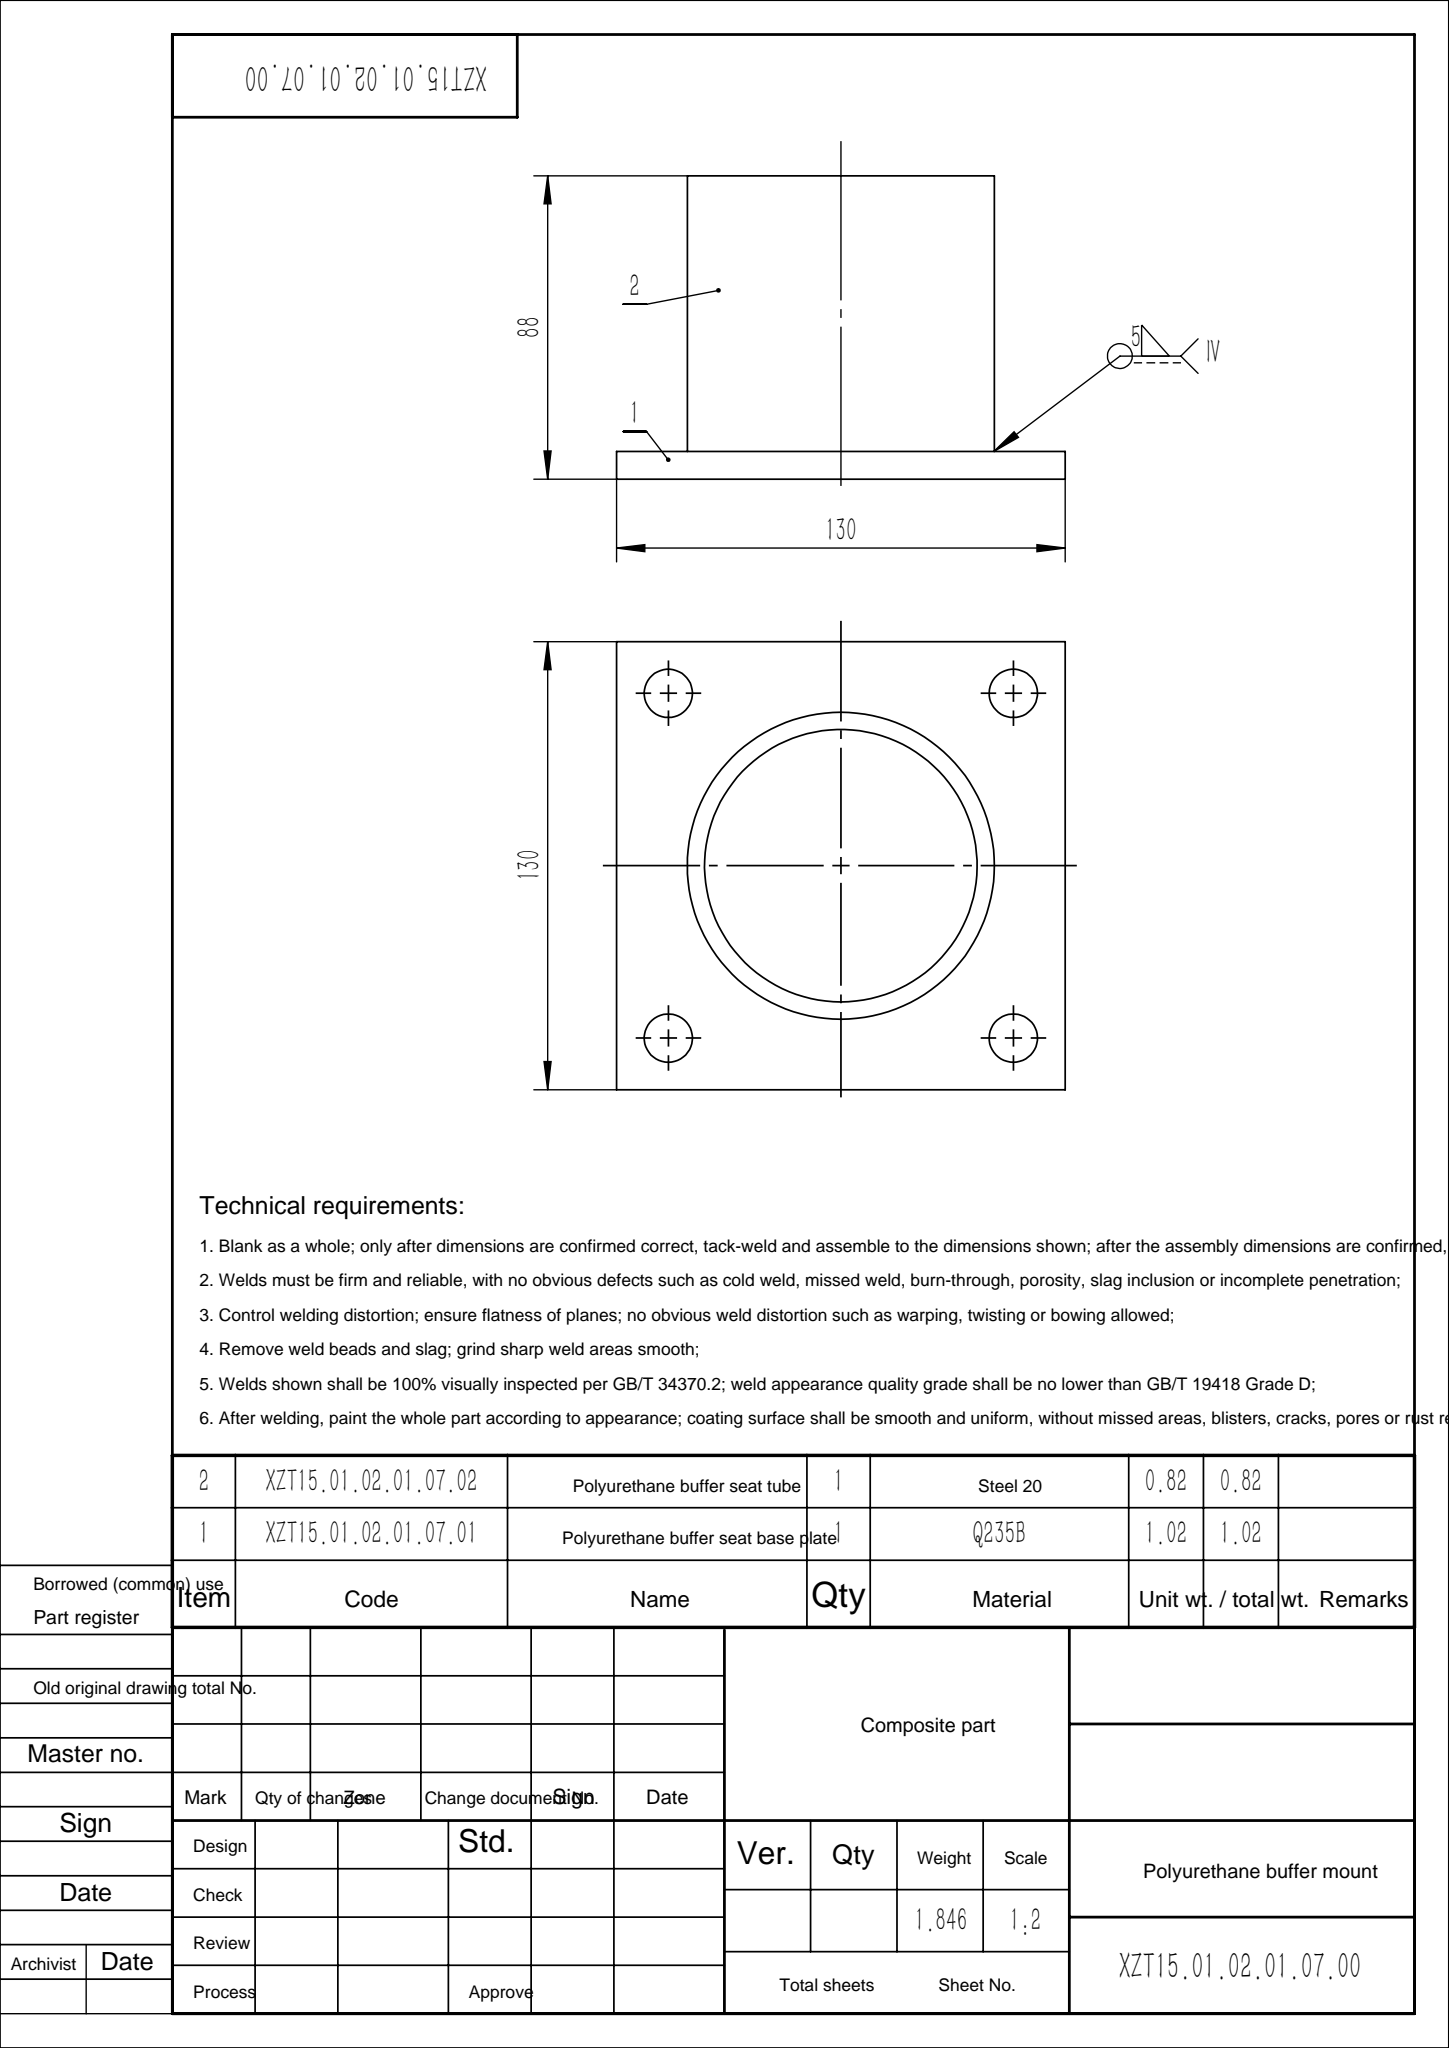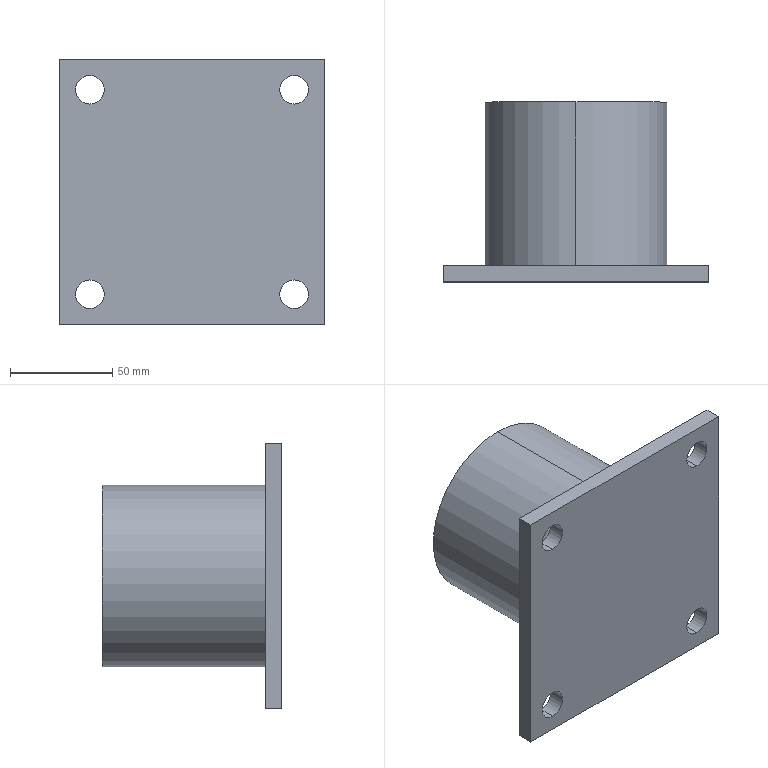Part | SolidWorks | 2 solids | 20 faces | box 130 x 88 x 130 mm | volume 235831 mm3 | cylinder 12 | plane 8 | commonest cylinder face diameters 14 x8 79 x2 89 x2